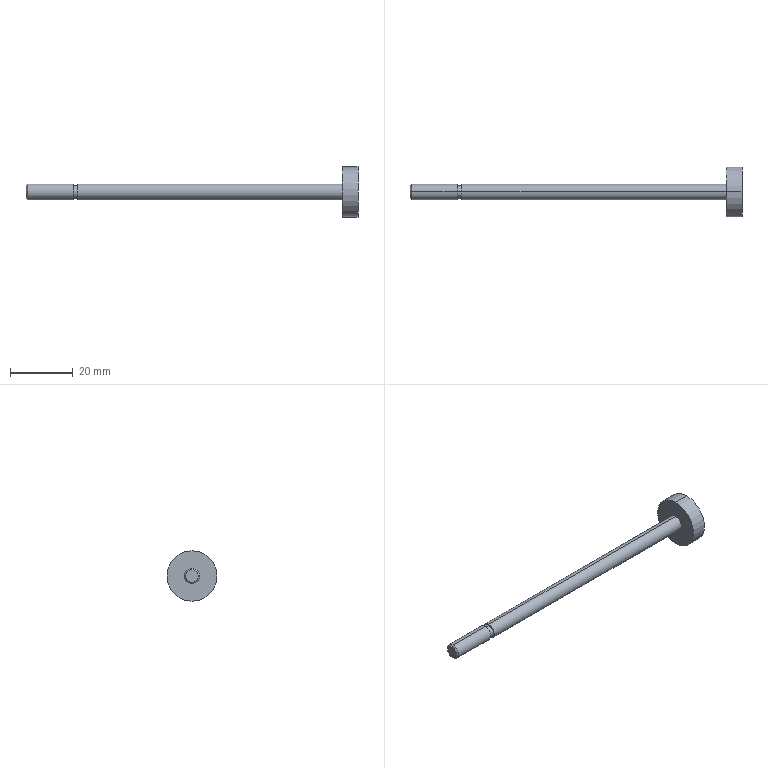Part | SolidWorks | features RefAxis 12, 3DProfileFeature 4, Revolution 1 | 1 solid | 15 faces | box 105.5 x 16 x 16 mm | volume 2967 mm3 | cylinder 8 | plane 5 | cone 2 | commonest cylinder face diameters 5 x4 4.13 x2 16 x2
STEP:
#1=CARTESIAN_POINT('',(105.5,0.,8.));
#2=VERTEX_POINT('',#1);
#3=CARTESIAN_POINT('',(105.5,0.,-8.));
#4=VERTEX_POINT('',#3);
#5=CARTESIAN_POINT('',(105.5,0.,0.));
#6=DIRECTION('',(-1.,0.,0.));
#7=DIRECTION('',(0.,0.,1.));
#8=AXIS2_PLACEMENT_3D('',#5,#6,#7);
#9=CIRCLE('',#8,8.);
#10=EDGE_CURVE('',#2,#4,#9,.T.);
#11=ORIENTED_EDGE('',*,*,#10,.T.);
#12=CARTESIAN_POINT('',(100.5,0.,-8.));
#13=VERTEX_POINT('',#12);
#14=CARTESIAN_POINT('',(105.5,0.,-8.));
#15=DIRECTION('',(-1.,0.,0.));
#16=VECTOR('',#15,1000.);
#17=LINE('',#14,#16);
#18=EDGE_CURVE('',#4,#13,#17,.T.);
#19=ORIENTED_EDGE('',*,*,#18,.T.);
#20=CARTESIAN_POINT('',(100.5,0.,8.));
#21=VERTEX_POINT('',#20);
#22=CARTESIAN_POINT('',(100.5,0.,0.));
#23=DIRECTION('',(-1.,0.,0.));
#24=DIRECTION('',(0.,0.,1.));
#25=AXIS2_PLACEMENT_3D('',#22,#23,#24);
#26=CIRCLE('',#25,8.);
#27=EDGE_CURVE('',#21,#13,#26,.T.);
#28=ORIENTED_EDGE('',*,*,#27,.F.);
#29=CARTESIAN_POINT('',(105.5,0.,8.));
#30=DIRECTION('',(-1.,0.,0.));
#31=VECTOR('',#30,1000.);
#32=LINE('',#29,#31);
#33=EDGE_CURVE('',#2,#21,#32,.T.);
#34=ORIENTED_EDGE('',*,*,#33,.F.);
#35=EDGE_LOOP('',(#11,#19,#28,#34));
#36=FACE_OUTER_BOUND('',#35,.T.);
#37=CARTESIAN_POINT('',(105.5,0.,0.));
#38=DIRECTION('',(-1.,0.,0.));
#39=DIRECTION('',(0.,0.,1.));
#40=AXIS2_PLACEMENT_3D('',#37,#38,#39);
#41=CYLINDRICAL_SURFACE('',#40,8.);
#42=ADVANCED_FACE('',(#36),#41,.T.);
#43=CARTESIAN_POINT('',(100.5,0.,2.5));
#44=VERTEX_POINT('',#43);
#45=CARTESIAN_POINT('',(100.5,0.,-2.5));
#46=VERTEX_POINT('',#45);
#47=CARTESIAN_POINT('',(100.5,0.,0.));
#48=DIRECTION('',(-1.,0.,0.));
#49=DIRECTION('',(0.,0.,1.));
#50=AXIS2_PLACEMENT_3D('',#47,#48,#49);
#51=CIRCLE('',#50,2.5);
#52=EDGE_CURVE('',#44,#46,#51,.T.);
#53=ORIENTED_EDGE('',*,*,#52,.T.);
#54=CARTESIAN_POINT('',(16.5,0.,-2.5));
#55=VERTEX_POINT('',#54);
#56=CARTESIAN_POINT('',(105.5,0.,-2.5));
#57=DIRECTION('',(-1.,0.,0.));
#58=VECTOR('',#57,1000.);
#59=LINE('',#56,#58);
#60=EDGE_CURVE('',#46,#55,#59,.T.);
#61=ORIENTED_EDGE('',*,*,#60,.T.);
#62=CARTESIAN_POINT('',(16.5,0.,2.5));
#63=VERTEX_POINT('',#62);
#64=CARTESIAN_POINT('',(16.5,0.,0.));
#65=DIRECTION('',(-1.,0.,0.));
#66=DIRECTION('',(0.,0.,1.));
#67=AXIS2_PLACEMENT_3D('',#64,#65,#66);
#68=CIRCLE('',#67,2.5);
#69=EDGE_CURVE('',#63,#55,#68,.T.);
#70=ORIENTED_EDGE('',*,*,#69,.F.);
#71=CARTESIAN_POINT('',(105.5,0.,2.5));
#72=DIRECTION('',(-1.,0.,0.));
#73=VECTOR('',#72,1000.);
#74=LINE('',#71,#73);
#75=EDGE_CURVE('',#44,#63,#74,.T.);
#76=ORIENTED_EDGE('',*,*,#75,.F.);
#77=EDGE_LOOP('',(#53,#61,#70,#76));
#78=FACE_OUTER_BOUND('',#77,.T.);
#79=CARTESIAN_POINT('',(105.5,0.,0.));
#80=DIRECTION('',(-1.,0.,0.));
#81=DIRECTION('',(0.,0.,1.));
#82=AXIS2_PLACEMENT_3D('',#79,#80,#81);
#83=CYLINDRICAL_SURFACE('',#82,2.5);
#84=ADVANCED_FACE('',(#78),#83,.T.);
#85=CARTESIAN_POINT('',(16.5,0.,2.065));
#86=VERTEX_POINT('',#85);
#87=CARTESIAN_POINT('',(16.5,0.,-2.065));
#88=VERTEX_POINT('',#87);
#89=CARTESIAN_POINT('',(16.5,0.,0.));
#90=DIRECTION('',(-1.,0.,0.));
#91=DIRECTION('',(0.,0.,1.));
#92=AXIS2_PLACEMENT_3D('',#89,#90,#91);
#93=CIRCLE('',#92,2.065);
#94=EDGE_CURVE('',#86,#88,#93,.T.);
#95=ORIENTED_EDGE('',*,*,#94,.T.);
#96=CARTESIAN_POINT('',(15.,0.,-2.065));
#97=VERTEX_POINT('',#96);
#98=CARTESIAN_POINT('',(105.5,0.,-2.065));
#99=DIRECTION('',(-1.,0.,0.));
#100=VECTOR('',#99,1000.);
#101=LINE('',#98,#100);
#102=EDGE_CURVE('',#88,#97,#101,.T.);
#103=ORIENTED_EDGE('',*,*,#102,.T.);
#104=CARTESIAN_POINT('',(15.,0.,2.065));
#105=VERTEX_POINT('',#104);
#106=CARTESIAN_POINT('',(15.,0.,0.));
#107=DIRECTION('',(-1.,0.,0.));
#108=DIRECTION('',(0.,0.,1.));
#109=AXIS2_PLACEMENT_3D('',#106,#107,#108);
#110=CIRCLE('',#109,2.065);
#111=EDGE_CURVE('',#105,#97,#110,.T.);
#112=ORIENTED_EDGE('',*,*,#111,.F.);
#113=CARTESIAN_POINT('',(105.5,0.,2.065));
#114=DIRECTION('',(-1.,0.,0.));
#115=VECTOR('',#114,1000.);
#116=LINE('',#113,#115);
#117=EDGE_CURVE('',#86,#105,#116,.T.);
#118=ORIENTED_EDGE('',*,*,#117,.F.);
#119=EDGE_LOOP('',(#95,#103,#112,#118));
#120=FACE_OUTER_BOUND('',#119,.T.);
#121=CARTESIAN_POINT('',(105.5,0.,0.));
#122=DIRECTION('',(-1.,0.,0.));
#123=DIRECTION('',(0.,0.,1.));
#124=AXIS2_PLACEMENT_3D('',#121,#122,#123);
#125=CYLINDRICAL_SURFACE('',#124,2.065);
#126=ADVANCED_FACE('',(#120),#125,.T.);
#127=CARTESIAN_POINT('',(15.,0.,2.5));
#128=VERTEX_POINT('',#127);
#129=CARTESIAN_POINT('',(15.,0.,-2.5));
#130=VERTEX_POINT('',#129);
#131=CARTESIAN_POINT('',(15.,0.,0.));
#132=DIRECTION('',(-1.,0.,0.));
#133=DIRECTION('',(0.,0.,1.));
#134=AXIS2_PLACEMENT_3D('',#131,#132,#133);
#135=CIRCLE('',#134,2.5);
#136=EDGE_CURVE('',#128,#130,#135,.T.);
#137=ORIENTED_EDGE('',*,*,#136,.T.);
#138=CARTESIAN_POINT('',(0.4905,0.,-2.5));
#139=VERTEX_POINT('',#138);
#140=CARTESIAN_POINT('',(105.5,0.,-2.5));
#141=DIRECTION('',(-1.,0.,0.));
#142=VECTOR('',#141,1000.);
#143=LINE('',#140,#142);
#144=EDGE_CURVE('',#130,#139,#143,.T.);
#145=ORIENTED_EDGE('',*,*,#144,.T.);
#146=CARTESIAN_POINT('',(0.4905,0.,2.5));
#147=VERTEX_POINT('',#146);
#148=CARTESIAN_POINT('',(0.4905,0.,0.));
#149=DIRECTION('',(-1.,0.,0.));
#150=DIRECTION('',(0.,0.,1.));
#151=AXIS2_PLACEMENT_3D('',#148,#149,#150);
#152=CIRCLE('',#151,2.5);
#153=EDGE_CURVE('',#147,#139,#152,.T.);
#154=ORIENTED_EDGE('',*,*,#153,.F.);
#155=CARTESIAN_POINT('',(105.5,0.,2.5));
#156=DIRECTION('',(-1.,0.,0.));
#157=VECTOR('',#156,1000.);
#158=LINE('',#155,#157);
#159=EDGE_CURVE('',#128,#147,#158,.T.);
#160=ORIENTED_EDGE('',*,*,#159,.F.);
#161=EDGE_LOOP('',(#137,#145,#154,#160));
#162=FACE_OUTER_BOUND('',#161,.T.);
#163=CARTESIAN_POINT('',(105.5,0.,0.));
#164=DIRECTION('',(-1.,0.,0.));
#165=DIRECTION('',(0.,0.,1.));
#166=AXIS2_PLACEMENT_3D('',#163,#164,#165);
#167=CYLINDRICAL_SURFACE('',#166,2.5);
#168=ADVANCED_FACE('',(#162),#167,.T.);
#169=CARTESIAN_POINT('',(0.,0.,2.01));
#170=VERTEX_POINT('',#169);
#171=CARTESIAN_POINT('',(0.,0.,-2.01));
#172=VERTEX_POINT('',#171);
#173=CARTESIAN_POINT('',(0.,0.,0.));
#174=DIRECTION('',(-1.,0.,0.));
#175=DIRECTION('',(0.,0.,1.));
#176=AXIS2_PLACEMENT_3D('',#173,#174,#175);
#177=CIRCLE('',#176,2.01);
#178=EDGE_CURVE('',#170,#172,#177,.T.);
#179=ORIENTED_EDGE('',*,*,#178,.F.);
#180=CARTESIAN_POINT('',(0.4905,0.,2.5));
#181=DIRECTION('',(0.7071,0.,0.7071));
#182=VECTOR('',#181,1000.);
#183=LINE('',#180,#182);
#184=EDGE_CURVE('',#170,#147,#183,.T.);
#185=ORIENTED_EDGE('',*,*,#184,.T.);
#186=ORIENTED_EDGE('',*,*,#153,.T.);
#187=CARTESIAN_POINT('',(0.4905,0.,-2.5));
#188=DIRECTION('',(0.7071,0.,-0.7071));
#189=VECTOR('',#188,1000.);
#190=LINE('',#187,#189);
#191=EDGE_CURVE('',#172,#139,#190,.T.);
#192=ORIENTED_EDGE('',*,*,#191,.F.);
#193=EDGE_LOOP('',(#179,#185,#186,#192));
#194=FACE_OUTER_BOUND('',#193,.T.);
#195=CARTESIAN_POINT('',(0.4905,0.,0.));
#196=DIRECTION('',(1.,0.,0.));
#197=DIRECTION('',(0.,0.,-1.));
#198=AXIS2_PLACEMENT_3D('',#195,#196,#197);
#199=CONICAL_SURFACE('',#198,2.5,0.7854);
#200=ADVANCED_FACE('',(#194),#199,.T.);
#201=CARTESIAN_POINT('',(0.,0.,0.));
#202=DIRECTION('',(-1.,0.,0.));
#203=DIRECTION('',(0.,0.,1.));
#204=AXIS2_PLACEMENT_3D('',#201,#202,#203);
#205=CIRCLE('',#204,2.01);
#206=EDGE_CURVE('',#172,#170,#205,.T.);
#207=ORIENTED_EDGE('',*,*,#206,.T.);
#208=ORIENTED_EDGE('',*,*,#178,.T.);
#209=EDGE_LOOP('',(#207,#208));
#210=FACE_OUTER_BOUND('',#209,.T.);
#211=CARTESIAN_POINT('',(0.,0.,0.));
#212=DIRECTION('',(1.,0.,0.));
#213=DIRECTION('',(0.,0.,-1.));
#214=AXIS2_PLACEMENT_3D('',#211,#212,#213);
#215=PLANE('',#214);
#216=ADVANCED_FACE('',(#210),#215,.F.);
#217=ORIENTED_EDGE('',*,*,#184,.F.);
#218=ORIENTED_EDGE('',*,*,#206,.F.);
#219=ORIENTED_EDGE('',*,*,#191,.T.);
#220=CARTESIAN_POINT('',(0.4905,0.,0.));
#221=DIRECTION('',(-1.,0.,0.));
#222=DIRECTION('',(0.,0.,1.));
#223=AXIS2_PLACEMENT_3D('',#220,#221,#222);
#224=CIRCLE('',#223,2.5);
#225=EDGE_CURVE('',#139,#147,#224,.T.);
#226=ORIENTED_EDGE('',*,*,#225,.T.);
#227=EDGE_LOOP('',(#217,#218,#219,#226));
#228=FACE_OUTER_BOUND('',#227,.T.);
#229=CARTESIAN_POINT('',(0.4905,0.,0.));
#230=DIRECTION('',(1.,0.,0.));
#231=DIRECTION('',(0.,0.,-1.));
#232=AXIS2_PLACEMENT_3D('',#229,#230,#231);
#233=CONICAL_SURFACE('',#232,2.5,0.7854);
#234=ADVANCED_FACE('',(#228),#233,.T.);
#235=ORIENTED_EDGE('',*,*,#144,.F.);
#236=CARTESIAN_POINT('',(15.,0.,0.));
#237=DIRECTION('',(-1.,0.,0.));
#238=DIRECTION('',(0.,0.,1.));
#239=AXIS2_PLACEMENT_3D('',#236,#237,#238);
#240=CIRCLE('',#239,2.5);
#241=EDGE_CURVE('',#130,#128,#240,.T.);
#242=ORIENTED_EDGE('',*,*,#241,.T.);
#243=ORIENTED_EDGE('',*,*,#159,.T.);
#244=ORIENTED_EDGE('',*,*,#225,.F.);
#245=EDGE_LOOP('',(#235,#242,#243,#244));
#246=FACE_OUTER_BOUND('',#245,.T.);
#247=CARTESIAN_POINT('',(105.5,0.,0.));
#248=DIRECTION('',(-1.,0.,0.));
#249=DIRECTION('',(0.,0.,1.));
#250=AXIS2_PLACEMENT_3D('',#247,#248,#249);
#251=CYLINDRICAL_SURFACE('',#250,2.5);
#252=ADVANCED_FACE('',(#246),#251,.T.);
#253=ORIENTED_EDGE('',*,*,#136,.F.);
#254=ORIENTED_EDGE('',*,*,#241,.F.);
#255=EDGE_LOOP('',(#253,#254));
#256=FACE_OUTER_BOUND('',#255,.T.);
#257=ORIENTED_EDGE('',*,*,#111,.T.);
#258=CARTESIAN_POINT('',(15.,0.,0.));
#259=DIRECTION('',(-1.,0.,0.));
#260=DIRECTION('',(0.,0.,1.));
#261=AXIS2_PLACEMENT_3D('',#258,#259,#260);
#262=CIRCLE('',#261,2.065);
#263=EDGE_CURVE('',#97,#105,#262,.T.);
#264=ORIENTED_EDGE('',*,*,#263,.T.);
#265=EDGE_LOOP('',(#257,#264));
#266=FACE_BOUND('',#265,.T.);
#267=CARTESIAN_POINT('',(15.,2.5,0.));
#268=DIRECTION('',(-1.,0.,0.));
#269=DIRECTION('',(0.,0.,1.));
#270=AXIS2_PLACEMENT_3D('',#267,#268,#269);
#271=PLANE('',#270);
#272=ADVANCED_FACE('',(#256,#266),#271,.F.);
#273=ORIENTED_EDGE('',*,*,#102,.F.);
#274=CARTESIAN_POINT('',(16.5,0.,0.));
#275=DIRECTION('',(-1.,0.,0.));
#276=DIRECTION('',(0.,0.,1.));
#277=AXIS2_PLACEMENT_3D('',#274,#275,#276);
#278=CIRCLE('',#277,2.065);
#279=EDGE_CURVE('',#88,#86,#278,.T.);
#280=ORIENTED_EDGE('',*,*,#279,.T.);
#281=ORIENTED_EDGE('',*,*,#117,.T.);
#282=ORIENTED_EDGE('',*,*,#263,.F.);
#283=EDGE_LOOP('',(#273,#280,#281,#282));
#284=FACE_OUTER_BOUND('',#283,.T.);
#285=CARTESIAN_POINT('',(105.5,0.,0.));
#286=DIRECTION('',(-1.,0.,0.));
#287=DIRECTION('',(0.,0.,1.));
#288=AXIS2_PLACEMENT_3D('',#285,#286,#287);
#289=CYLINDRICAL_SURFACE('',#288,2.065);
#290=ADVANCED_FACE('',(#284),#289,.T.);
#291=ORIENTED_EDGE('',*,*,#94,.F.);
#292=ORIENTED_EDGE('',*,*,#279,.F.);
#293=EDGE_LOOP('',(#291,#292));
#294=FACE_BOUND('',#293,.T.);
#295=ORIENTED_EDGE('',*,*,#69,.T.);
#296=CARTESIAN_POINT('',(16.5,0.,0.));
#297=DIRECTION('',(-1.,0.,0.));
#298=DIRECTION('',(0.,0.,1.));
#299=AXIS2_PLACEMENT_3D('',#296,#297,#298);
#300=CIRCLE('',#299,2.5);
#301=EDGE_CURVE('',#55,#63,#300,.T.);
#302=ORIENTED_EDGE('',*,*,#301,.T.);
#303=EDGE_LOOP('',(#295,#302));
#304=FACE_OUTER_BOUND('',#303,.T.);
#305=CARTESIAN_POINT('',(16.5,2.065,0.));
#306=DIRECTION('',(1.,0.,0.));
#307=DIRECTION('',(0.,0.,-1.));
#308=AXIS2_PLACEMENT_3D('',#305,#306,#307);
#309=PLANE('',#308);
#310=ADVANCED_FACE('',(#294,#304),#309,.F.);
#311=ORIENTED_EDGE('',*,*,#60,.F.);
#312=CARTESIAN_POINT('',(100.5,0.,0.));
#313=DIRECTION('',(-1.,0.,0.));
#314=DIRECTION('',(0.,0.,1.));
#315=AXIS2_PLACEMENT_3D('',#312,#313,#314);
#316=CIRCLE('',#315,2.5);
#317=EDGE_CURVE('',#46,#44,#316,.T.);
#318=ORIENTED_EDGE('',*,*,#317,.T.);
#319=ORIENTED_EDGE('',*,*,#75,.T.);
#320=ORIENTED_EDGE('',*,*,#301,.F.);
#321=EDGE_LOOP('',(#311,#318,#319,#320));
#322=FACE_OUTER_BOUND('',#321,.T.);
#323=CARTESIAN_POINT('',(105.5,0.,0.));
#324=DIRECTION('',(-1.,0.,0.));
#325=DIRECTION('',(0.,0.,1.));
#326=AXIS2_PLACEMENT_3D('',#323,#324,#325);
#327=CYLINDRICAL_SURFACE('',#326,2.5);
#328=ADVANCED_FACE('',(#322),#327,.T.);
#329=ORIENTED_EDGE('',*,*,#52,.F.);
#330=ORIENTED_EDGE('',*,*,#317,.F.);
#331=EDGE_LOOP('',(#329,#330));
#332=FACE_BOUND('',#331,.T.);
#333=ORIENTED_EDGE('',*,*,#27,.T.);
#334=CARTESIAN_POINT('',(100.5,0.,0.));
#335=DIRECTION('',(-1.,0.,0.));
#336=DIRECTION('',(0.,0.,1.));
#337=AXIS2_PLACEMENT_3D('',#334,#335,#336);
#338=CIRCLE('',#337,8.);
#339=EDGE_CURVE('',#13,#21,#338,.T.);
#340=ORIENTED_EDGE('',*,*,#339,.T.);
#341=EDGE_LOOP('',(#333,#340));
#342=FACE_OUTER_BOUND('',#341,.T.);
#343=CARTESIAN_POINT('',(100.5,2.5,0.));
#344=DIRECTION('',(1.,0.,0.));
#345=DIRECTION('',(0.,0.,-1.));
#346=AXIS2_PLACEMENT_3D('',#343,#344,#345);
#347=PLANE('',#346);
#348=ADVANCED_FACE('',(#332,#342),#347,.F.);
#349=ORIENTED_EDGE('',*,*,#18,.F.);
#350=CARTESIAN_POINT('',(105.5,0.,0.));
#351=DIRECTION('',(-1.,0.,0.));
#352=DIRECTION('',(0.,0.,1.));
#353=AXIS2_PLACEMENT_3D('',#350,#351,#352);
#354=CIRCLE('',#353,8.);
#355=EDGE_CURVE('',#4,#2,#354,.T.);
#356=ORIENTED_EDGE('',*,*,#355,.T.);
#357=ORIENTED_EDGE('',*,*,#33,.T.);
#358=ORIENTED_EDGE('',*,*,#339,.F.);
#359=EDGE_LOOP('',(#349,#356,#357,#358));
#360=FACE_OUTER_BOUND('',#359,.T.);
#361=CARTESIAN_POINT('',(105.5,0.,0.));
#362=DIRECTION('',(-1.,0.,0.));
#363=DIRECTION('',(0.,0.,1.));
#364=AXIS2_PLACEMENT_3D('',#361,#362,#363);
#365=CYLINDRICAL_SURFACE('',#364,8.);
#366=ADVANCED_FACE('',(#360),#365,.T.);
#367=ORIENTED_EDGE('',*,*,#10,.F.);
#368=ORIENTED_EDGE('',*,*,#355,.F.);
#369=EDGE_LOOP('',(#367,#368));
#370=FACE_OUTER_BOUND('',#369,.T.);
#371=CARTESIAN_POINT('',(105.5,8.,0.));
#372=DIRECTION('',(-1.,0.,0.));
#373=DIRECTION('',(0.,0.,1.));
#374=AXIS2_PLACEMENT_3D('',#371,#372,#373);
#375=PLANE('',#374);
#376=ADVANCED_FACE('',(#370),#375,.F.);
#377=CLOSED_SHELL('',(#42,#84,#126,#168,#200,#216,#234,#252,#272,#290,#310,#328,#348,#366,#376));
#378=MANIFOLD_SOLID_BREP('',#377);
#379=CARTESIAN_POINT('',(0.,0.,0.));
#380=DIRECTION('',(0.,0.,1.));
#381=DIRECTION('',(1.,0.,0.));
#382=AXIS2_PLACEMENT_3D('',#379,#380,#381);
#383=(LENGTH_UNIT()NAMED_UNIT(*)SI_UNIT(.MILLI.,.METRE.));
#384=UNCERTAINTY_MEASURE_WITH_UNIT(LENGTH_MEASURE(0.00001),#383,'','');
#385=(NAMED_UNIT(*)PLANE_ANGLE_UNIT()SI_UNIT($,.RADIAN.));
#386=(NAMED_UNIT(*)SI_UNIT($,.STERADIAN.)SOLID_ANGLE_UNIT());
#387=(GEOMETRIC_REPRESENTATION_CONTEXT(3)GLOBAL_UNCERTAINTY_ASSIGNED_CONTEXT((#384))GLOBAL_UNIT_ASSIGNED_CONTEXT((#383,#385,#386))REPRESENTATION_CONTEXT('',''));
#388=ADVANCED_BREP_SHAPE_REPRESENTATION('',(#378,#382),#387);